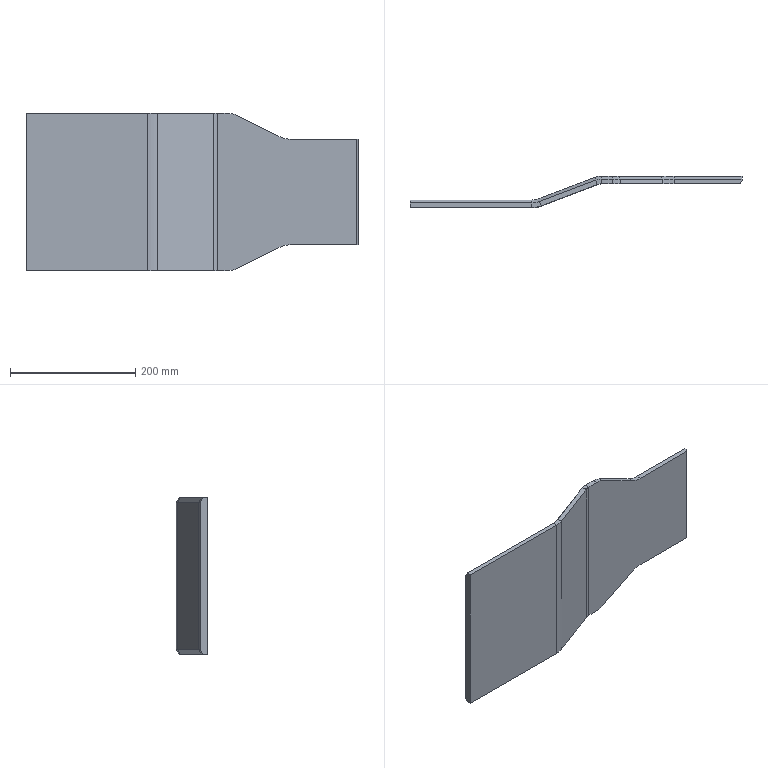Part | SolidWorks | features Chamfer 2, Cut 1, Extrusion 1, FlatPattern 1, SheetMetal 1, SolidToSheetMetal 1 | 1 solid | 49 faces | box 530 x 50 x 251 mm | volume 1438713 mm3 | plane 33 | cylinder 8 | cone 8 | commonest cylinder face diameters 60 x4 80 x2 36 x1 84 x1
STEP:
#1=CARTESIAN_POINT('',(0.,-50.,-10.));
#2=VERTEX_POINT('',#1);
#3=CARTESIAN_POINT('',(0.,-42.619,-10.));
#4=VERTEX_POINT('',#3);
#5=CARTESIAN_POINT('',(0.,-38.,-10.));
#6=DIRECTION('',(0.,1.,0.));
#7=VECTOR('',#6,1000.);
#8=LINE('',#5,#7);
#9=EDGE_CURVE('',#2,#4,#8,.T.);
#10=ORIENTED_EDGE('',*,*,#9,.T.);
#11=CARTESIAN_POINT('',(0.,-38.,-18.));
#12=VERTEX_POINT('',#11);
#13=CARTESIAN_POINT('',(0.,297.738,-599.515));
#14=DIRECTION('',(0.,0.5,-0.866));
#15=VECTOR('',#14,1000.);
#16=LINE('',#13,#15);
#17=EDGE_CURVE('',#4,#12,#16,.T.);
#18=ORIENTED_EDGE('',*,*,#17,.T.);
#19=CARTESIAN_POINT('',(0.,-38.,-253.));
#20=VERTEX_POINT('',#19);
#21=CARTESIAN_POINT('',(0.,-38.,-793.353));
#22=DIRECTION('',(0.,0.,1.));
#23=VECTOR('',#22,1000.);
#24=LINE('',#21,#23);
#25=EDGE_CURVE('',#20,#12,#24,.T.);
#26=ORIENTED_EDGE('',*,*,#25,.F.);
#27=CARTESIAN_POINT('',(0.,-42.619,-261.));
#28=VERTEX_POINT('',#27);
#29=CARTESIAN_POINT('',(0.,-271.98,-658.265));
#30=DIRECTION('',(0.,-0.5,-0.866));
#31=VECTOR('',#30,1000.);
#32=LINE('',#29,#31);
#33=EDGE_CURVE('',#20,#28,#32,.T.);
#34=ORIENTED_EDGE('',*,*,#33,.T.);
#35=CARTESIAN_POINT('',(0.,-50.,-261.));
#36=VERTEX_POINT('',#35);
#37=CARTESIAN_POINT('',(0.,-38.,-261.));
#38=DIRECTION('',(0.,1.,0.));
#39=VECTOR('',#38,1000.);
#40=LINE('',#37,#39);
#41=EDGE_CURVE('',#36,#28,#40,.T.);
#42=ORIENTED_EDGE('',*,*,#41,.F.);
#43=CARTESIAN_POINT('',(0.,-50.,-793.353));
#44=DIRECTION('',(0.,0.,1.));
#45=VECTOR('',#44,1000.);
#46=LINE('',#43,#45);
#47=EDGE_CURVE('',#36,#2,#46,.T.);
#48=ORIENTED_EDGE('',*,*,#47,.T.);
#49=EDGE_LOOP('',(#10,#18,#26,#34,#42,#48));
#50=FACE_OUTER_BOUND('',#49,.T.);
#51=CARTESIAN_POINT('',(0.,-38.,-793.353));
#52=DIRECTION('',(-1.,0.,0.));
#53=DIRECTION('',(0.,0.,1.));
#54=AXIS2_PLACEMENT_3D('',#51,#52,#53);
#55=PLANE('',#54);
#56=ADVANCED_FACE('',(#50),#55,.T.);
#57=CARTESIAN_POINT('',(194.492,-50.,-10.));
#58=VERTEX_POINT('',#57);
#59=CARTESIAN_POINT('',(194.492,-42.619,-10.));
#60=VERTEX_POINT('',#59);
#61=CARTESIAN_POINT('',(194.492,-38.,-10.));
#62=DIRECTION('',(0.,1.,0.));
#63=VECTOR('',#62,1000.);
#64=LINE('',#61,#63);
#65=EDGE_CURVE('',#58,#60,#64,.T.);
#66=ORIENTED_EDGE('',*,*,#65,.T.);
#67=CARTESIAN_POINT('',(0.,-42.619,-10.));
#68=DIRECTION('',(-1.,0.,0.));
#69=VECTOR('',#68,1000.);
#70=LINE('',#67,#69);
#71=EDGE_CURVE('',#60,#4,#70,.T.);
#72=ORIENTED_EDGE('',*,*,#71,.T.);
#73=ORIENTED_EDGE('',*,*,#9,.F.);
#74=CARTESIAN_POINT('',(0.,-50.,-10.));
#75=DIRECTION('',(-1.,0.,0.));
#76=VECTOR('',#75,1000.);
#77=LINE('',#74,#76);
#78=EDGE_CURVE('',#58,#2,#77,.T.);
#79=ORIENTED_EDGE('',*,*,#78,.F.);
#80=EDGE_LOOP('',(#66,#72,#73,#79));
#81=FACE_OUTER_BOUND('',#80,.T.);
#82=CARTESIAN_POINT('',(0.,-38.,-10.));
#83=DIRECTION('',(0.,0.,-1.));
#84=DIRECTION('',(-1.,0.,0.));
#85=AXIS2_PLACEMENT_3D('',#82,#83,#84);
#86=PLANE('',#85);
#87=ADVANCED_FACE('',(#81),#86,.F.);
#88=CARTESIAN_POINT('',(209.411,-47.261,-10.));
#89=VERTEX_POINT('',#88);
#90=CARTESIAN_POINT('',(206.789,-40.361,-10.));
#91=VERTEX_POINT('',#90);
#92=CARTESIAN_POINT('',(205.149,-36.044,-10.));
#93=DIRECTION('',(-0.3552,0.9348,0.));
#94=VECTOR('',#93,1000.);
#95=LINE('',#92,#94);
#96=EDGE_CURVE('',#89,#91,#95,.T.);
#97=ORIENTED_EDGE('',*,*,#96,.T.);
#98=CARTESIAN_POINT('',(194.492,-8.,-10.));
#99=DIRECTION('',(0.,0.,-1.));
#100=DIRECTION('',(1.,0.,0.));
#101=AXIS2_PLACEMENT_3D('',#98,#99,#100);
#102=CIRCLE('',#101,34.619);
#103=EDGE_CURVE('',#91,#60,#102,.T.);
#104=ORIENTED_EDGE('',*,*,#103,.T.);
#105=ORIENTED_EDGE('',*,*,#65,.F.);
#106=CARTESIAN_POINT('',(194.492,-8.,-10.));
#107=DIRECTION('',(0.,0.,-1.));
#108=DIRECTION('',(1.,0.,0.));
#109=AXIS2_PLACEMENT_3D('',#106,#107,#108);
#110=CIRCLE('',#109,42.);
#111=EDGE_CURVE('',#89,#58,#110,.T.);
#112=ORIENTED_EDGE('',*,*,#111,.F.);
#113=EDGE_LOOP('',(#97,#104,#105,#112));
#114=FACE_OUTER_BOUND('',#113,.T.);
#115=CARTESIAN_POINT('',(194.492,-8.,-10.));
#116=DIRECTION('',(0.,0.,1.));
#117=DIRECTION('',(1.,0.,0.));
#118=AXIS2_PLACEMENT_3D('',#115,#116,#117);
#119=PLANE('',#118);
#120=ADVANCED_FACE('',(#114),#119,.T.);
#121=CARTESIAN_POINT('',(299.114,-13.174,-10.));
#122=VERTEX_POINT('',#121);
#123=CARTESIAN_POINT('',(296.492,-6.274,-10.));
#124=VERTEX_POINT('',#123);
#125=CARTESIAN_POINT('',(294.851,-1.956,-10.));
#126=DIRECTION('',(-0.3552,0.9348,0.));
#127=VECTOR('',#126,1000.);
#128=LINE('',#125,#127);
#129=EDGE_CURVE('',#122,#124,#128,.T.);
#130=ORIENTED_EDGE('',*,*,#129,.T.);
#131=CARTESIAN_POINT('',(206.789,-40.361,-10.));
#132=DIRECTION('',(-0.9348,-0.3552,0.));
#133=VECTOR('',#132,1000.);
#134=LINE('',#131,#133);
#135=EDGE_CURVE('',#124,#91,#134,.T.);
#136=ORIENTED_EDGE('',*,*,#135,.T.);
#137=ORIENTED_EDGE('',*,*,#96,.F.);
#138=CARTESIAN_POINT('',(209.411,-47.261,-10.));
#139=DIRECTION('',(-0.9348,-0.3552,0.));
#140=VECTOR('',#139,1000.);
#141=LINE('',#138,#140);
#142=EDGE_CURVE('',#122,#89,#141,.T.);
#143=ORIENTED_EDGE('',*,*,#142,.F.);
#144=EDGE_LOOP('',(#130,#136,#137,#143));
#145=FACE_OUTER_BOUND('',#144,.T.);
#146=CARTESIAN_POINT('',(205.149,-36.044,-10.));
#147=DIRECTION('',(0.,0.,-1.));
#148=DIRECTION('',(-0.9348,-0.3552,0.));
#149=AXIS2_PLACEMENT_3D('',#146,#147,#148);
#150=PLANE('',#149);
#151=ADVANCED_FACE('',(#145),#150,.F.);
#152=CARTESIAN_POINT('',(305.508,-12.,-10.));
#153=VERTEX_POINT('',#152);
#154=CARTESIAN_POINT('',(305.508,-4.619,-10.));
#155=VERTEX_POINT('',#154);
#156=CARTESIAN_POINT('',(305.508,0.,-10.));
#157=DIRECTION('',(0.,1.,0.));
#158=VECTOR('',#157,1000.);
#159=LINE('',#156,#158);
#160=EDGE_CURVE('',#153,#155,#159,.T.);
#161=ORIENTED_EDGE('',*,*,#160,.T.);
#162=CARTESIAN_POINT('',(305.508,-30.,-10.));
#163=DIRECTION('',(0.,0.,1.));
#164=DIRECTION('',(-1.,0.,0.));
#165=AXIS2_PLACEMENT_3D('',#162,#163,#164);
#166=CIRCLE('',#165,25.381);
#167=EDGE_CURVE('',#155,#124,#166,.T.);
#168=ORIENTED_EDGE('',*,*,#167,.T.);
#169=ORIENTED_EDGE('',*,*,#129,.F.);
#170=CARTESIAN_POINT('',(305.508,-30.,-10.));
#171=DIRECTION('',(0.,0.,1.));
#172=DIRECTION('',(1.,0.,0.));
#173=AXIS2_PLACEMENT_3D('',#170,#171,#172);
#174=CIRCLE('',#173,18.);
#175=EDGE_CURVE('',#153,#122,#174,.T.);
#176=ORIENTED_EDGE('',*,*,#175,.F.);
#177=EDGE_LOOP('',(#161,#168,#169,#176));
#178=FACE_OUTER_BOUND('',#177,.T.);
#179=CARTESIAN_POINT('',(305.508,-30.,-10.));
#180=DIRECTION('',(0.,0.,-1.));
#181=DIRECTION('',(-1.,0.,0.));
#182=AXIS2_PLACEMENT_3D('',#179,#180,#181);
#183=PLANE('',#182);
#184=ADVANCED_FACE('',(#178),#183,.F.);
#185=CARTESIAN_POINT('',(322.918,-12.,-10.));
#186=VERTEX_POINT('',#185);
#187=CARTESIAN_POINT('',(322.918,-4.619,-10.));
#188=VERTEX_POINT('',#187);
#189=CARTESIAN_POINT('',(322.918,0.,-10.));
#190=DIRECTION('',(0.,1.,0.));
#191=VECTOR('',#190,1000.);
#192=LINE('',#189,#191);
#193=EDGE_CURVE('',#186,#188,#192,.T.);
#194=ORIENTED_EDGE('',*,*,#193,.T.);
#195=CARTESIAN_POINT('',(322.918,-4.619,-10.));
#196=DIRECTION('',(-1.,0.,0.));
#197=VECTOR('',#196,1000.);
#198=LINE('',#195,#197);
#199=EDGE_CURVE('',#188,#155,#198,.T.);
#200=ORIENTED_EDGE('',*,*,#199,.T.);
#201=ORIENTED_EDGE('',*,*,#160,.F.);
#202=CARTESIAN_POINT('',(322.918,-12.,-10.));
#203=DIRECTION('',(-1.,0.,0.));
#204=VECTOR('',#203,1000.);
#205=LINE('',#202,#204);
#206=EDGE_CURVE('',#186,#153,#205,.T.);
#207=ORIENTED_EDGE('',*,*,#206,.F.);
#208=EDGE_LOOP('',(#194,#200,#201,#207));
#209=FACE_OUTER_BOUND('',#208,.T.);
#210=CARTESIAN_POINT('',(322.918,0.,-10.));
#211=DIRECTION('',(0.,0.,-1.));
#212=DIRECTION('',(-1.,0.,0.));
#213=AXIS2_PLACEMENT_3D('',#210,#211,#212);
#214=PLANE('',#213);
#215=ADVANCED_FACE('',(#209),#214,.F.);
#216=CARTESIAN_POINT('',(336.334,-12.,-13.167));
#217=VERTEX_POINT('',#216);
#218=CARTESIAN_POINT('',(336.334,-4.619,-13.167));
#219=VERTEX_POINT('',#218);
#220=CARTESIAN_POINT('',(336.334,0.,-13.167));
#221=DIRECTION('',(0.,1.,0.));
#222=VECTOR('',#221,1000.);
#223=LINE('',#220,#222);
#224=EDGE_CURVE('',#217,#219,#223,.T.);
#225=ORIENTED_EDGE('',*,*,#224,.T.);
#226=CARTESIAN_POINT('',(322.918,-4.619,-40.));
#227=DIRECTION('',(0.,-1.,0.));
#228=DIRECTION('',(0.,0.,1.));
#229=AXIS2_PLACEMENT_3D('',#226,#227,#228);
#230=CIRCLE('',#229,30.);
#231=EDGE_CURVE('',#219,#188,#230,.T.);
#232=ORIENTED_EDGE('',*,*,#231,.T.);
#233=ORIENTED_EDGE('',*,*,#193,.F.);
#234=CARTESIAN_POINT('',(322.918,-12.,-40.));
#235=DIRECTION('',(0.,-1.,0.));
#236=DIRECTION('',(0.,0.,-1.));
#237=AXIS2_PLACEMENT_3D('',#234,#235,#236);
#238=CIRCLE('',#237,30.);
#239=EDGE_CURVE('',#217,#186,#238,.T.);
#240=ORIENTED_EDGE('',*,*,#239,.F.);
#241=EDGE_LOOP('',(#225,#232,#233,#240));
#242=FACE_OUTER_BOUND('',#241,.T.);
#243=CARTESIAN_POINT('',(322.918,0.,-40.));
#244=DIRECTION('',(0.,1.,0.));
#245=DIRECTION('',(0.,0.,1.));
#246=AXIS2_PLACEMENT_3D('',#243,#244,#245);
#247=CYLINDRICAL_SURFACE('',#246,30.);
#248=ADVANCED_FACE('',(#242),#247,.T.);
#249=CARTESIAN_POINT('',(403.666,-12.,-46.833));
#250=VERTEX_POINT('',#249);
#251=CARTESIAN_POINT('',(403.666,-4.619,-46.833));
#252=VERTEX_POINT('',#251);
#253=CARTESIAN_POINT('',(403.666,0.,-46.833));
#254=DIRECTION('',(0.,1.,0.));
#255=VECTOR('',#254,1000.);
#256=LINE('',#253,#255);
#257=EDGE_CURVE('',#250,#252,#256,.T.);
#258=ORIENTED_EDGE('',*,*,#257,.T.);
#259=CARTESIAN_POINT('',(403.666,-4.619,-46.833));
#260=DIRECTION('',(-0.8944,0.,0.4472));
#261=VECTOR('',#260,1000.);
#262=LINE('',#259,#261);
#263=EDGE_CURVE('',#252,#219,#262,.T.);
#264=ORIENTED_EDGE('',*,*,#263,.T.);
#265=ORIENTED_EDGE('',*,*,#224,.F.);
#266=CARTESIAN_POINT('',(403.666,-12.,-46.833));
#267=DIRECTION('',(-0.8944,0.,0.4472));
#268=VECTOR('',#267,1000.);
#269=LINE('',#266,#268);
#270=EDGE_CURVE('',#250,#217,#269,.T.);
#271=ORIENTED_EDGE('',*,*,#270,.F.);
#272=EDGE_LOOP('',(#258,#264,#265,#271));
#273=FACE_OUTER_BOUND('',#272,.T.);
#274=CARTESIAN_POINT('',(403.666,0.,-46.833));
#275=DIRECTION('',(-0.4472,0.,-0.8944));
#276=DIRECTION('',(-0.8944,0.,0.4472));
#277=AXIS2_PLACEMENT_3D('',#274,#275,#276);
#278=PLANE('',#277);
#279=ADVANCED_FACE('',(#273),#278,.F.);
#280=CARTESIAN_POINT('',(421.554,-12.,-51.056));
#281=VERTEX_POINT('',#280);
#282=CARTESIAN_POINT('',(421.554,-4.619,-51.056));
#283=VERTEX_POINT('',#282);
#284=CARTESIAN_POINT('',(421.554,0.,-51.056));
#285=DIRECTION('',(0.,1.,0.));
#286=VECTOR('',#285,1000.);
#287=LINE('',#284,#286);
#288=EDGE_CURVE('',#281,#283,#287,.T.);
#289=ORIENTED_EDGE('',*,*,#288,.T.);
#290=CARTESIAN_POINT('',(421.554,-4.619,-11.056));
#291=DIRECTION('',(0.,1.,0.));
#292=DIRECTION('',(0.,0.,1.));
#293=AXIS2_PLACEMENT_3D('',#290,#291,#292);
#294=CIRCLE('',#293,40.);
#295=EDGE_CURVE('',#283,#252,#294,.T.);
#296=ORIENTED_EDGE('',*,*,#295,.T.);
#297=ORIENTED_EDGE('',*,*,#257,.F.);
#298=CARTESIAN_POINT('',(421.554,-12.,-11.056));
#299=DIRECTION('',(0.,1.,0.));
#300=DIRECTION('',(0.,0.,1.));
#301=AXIS2_PLACEMENT_3D('',#298,#299,#300);
#302=CIRCLE('',#301,40.);
#303=EDGE_CURVE('',#281,#250,#302,.T.);
#304=ORIENTED_EDGE('',*,*,#303,.F.);
#305=EDGE_LOOP('',(#289,#296,#297,#304));
#306=FACE_OUTER_BOUND('',#305,.T.);
#307=CARTESIAN_POINT('',(421.554,0.,-11.056));
#308=DIRECTION('',(0.,1.,0.));
#309=DIRECTION('',(0.,0.,1.));
#310=AXIS2_PLACEMENT_3D('',#307,#308,#309);
#311=CYLINDRICAL_SURFACE('',#310,40.);
#312=ADVANCED_FACE('',(#306),#311,.F.);
#313=CARTESIAN_POINT('',(527.113,-12.,-51.056));
#314=VERTEX_POINT('',#313);
#315=CARTESIAN_POINT('',(322.918,-12.,-51.056));
#316=DIRECTION('',(-1.,0.,0.));
#317=VECTOR('',#316,1000.);
#318=LINE('',#315,#317);
#319=EDGE_CURVE('',#314,#281,#318,.T.);
#320=ORIENTED_EDGE('',*,*,#319,.F.);
#321=CARTESIAN_POINT('',(530.,-7.,-51.056));
#322=VERTEX_POINT('',#321);
#323=CARTESIAN_POINT('',(533.031,-1.75,-51.056));
#324=DIRECTION('',(0.5,0.866,0.));
#325=VECTOR('',#324,1000.);
#326=LINE('',#323,#325);
#327=EDGE_CURVE('',#314,#322,#326,.T.);
#328=ORIENTED_EDGE('',*,*,#327,.T.);
#329=CARTESIAN_POINT('',(530.,-4.619,-51.056));
#330=VERTEX_POINT('',#329);
#331=CARTESIAN_POINT('',(530.,0.,-51.056));
#332=DIRECTION('',(0.,1.,0.));
#333=VECTOR('',#332,1000.);
#334=LINE('',#331,#333);
#335=EDGE_CURVE('',#322,#330,#334,.T.);
#336=ORIENTED_EDGE('',*,*,#335,.T.);
#337=CARTESIAN_POINT('',(530.,-4.619,-51.056));
#338=DIRECTION('',(-1.,0.,0.));
#339=VECTOR('',#338,1000.);
#340=LINE('',#337,#339);
#341=EDGE_CURVE('',#330,#283,#340,.T.);
#342=ORIENTED_EDGE('',*,*,#341,.T.);
#343=ORIENTED_EDGE('',*,*,#288,.F.);
#344=EDGE_LOOP('',(#320,#328,#336,#342,#343));
#345=FACE_OUTER_BOUND('',#344,.T.);
#346=CARTESIAN_POINT('',(530.,0.,-51.056));
#347=DIRECTION('',(0.,0.,-1.));
#348=DIRECTION('',(-1.,0.,0.));
#349=AXIS2_PLACEMENT_3D('',#346,#347,#348);
#350=PLANE('',#349);
#351=ADVANCED_FACE('',(#345),#350,.F.);
#352=ORIENTED_EDGE('',*,*,#335,.F.);
#353=CARTESIAN_POINT('',(530.,-7.,-219.944));
#354=VERTEX_POINT('',#353);
#355=CARTESIAN_POINT('',(530.,-7.,-219.944));
#356=DIRECTION('',(0.,0.,-1.));
#357=VECTOR('',#356,1000.);
#358=LINE('',#355,#357);
#359=EDGE_CURVE('',#322,#354,#358,.T.);
#360=ORIENTED_EDGE('',*,*,#359,.T.);
#361=CARTESIAN_POINT('',(530.,-4.619,-219.944));
#362=VERTEX_POINT('',#361);
#363=CARTESIAN_POINT('',(530.,0.,-219.944));
#364=DIRECTION('',(0.,1.,0.));
#365=VECTOR('',#364,1000.);
#366=LINE('',#363,#365);
#367=EDGE_CURVE('',#354,#362,#366,.T.);
#368=ORIENTED_EDGE('',*,*,#367,.T.);
#369=CARTESIAN_POINT('',(530.,0.,-211.944));
#370=VERTEX_POINT('',#369);
#371=CARTESIAN_POINT('',(530.,-251.757,-648.001));
#372=DIRECTION('',(0.,0.5,0.866));
#373=VECTOR('',#372,1000.);
#374=LINE('',#371,#373);
#375=EDGE_CURVE('',#362,#370,#374,.T.);
#376=ORIENTED_EDGE('',*,*,#375,.T.);
#377=CARTESIAN_POINT('',(530.,0.,-59.056));
#378=VERTEX_POINT('',#377);
#379=CARTESIAN_POINT('',(530.,0.,-793.353));
#380=DIRECTION('',(0.,0.,1.));
#381=VECTOR('',#380,1000.);
#382=LINE('',#379,#381);
#383=EDGE_CURVE('',#370,#378,#382,.T.);
#384=ORIENTED_EDGE('',*,*,#383,.T.);
#385=CARTESIAN_POINT('',(530.,317.96,-609.779));
#386=DIRECTION('',(0.,-0.5,0.866));
#387=VECTOR('',#386,1000.);
#388=LINE('',#385,#387);
#389=EDGE_CURVE('',#378,#330,#388,.T.);
#390=ORIENTED_EDGE('',*,*,#389,.T.);
#391=EDGE_LOOP('',(#352,#360,#368,#376,#384,#390));
#392=FACE_OUTER_BOUND('',#391,.T.);
#393=CARTESIAN_POINT('',(530.,0.,-793.353));
#394=DIRECTION('',(-1.,0.,0.));
#395=DIRECTION('',(0.,0.,1.));
#396=AXIS2_PLACEMENT_3D('',#393,#394,#395);
#397=PLANE('',#396);
#398=ADVANCED_FACE('',(#392),#397,.F.);
#399=ORIENTED_EDGE('',*,*,#367,.F.);
#400=CARTESIAN_POINT('',(527.113,-12.,-219.944));
#401=VERTEX_POINT('',#400);
#402=CARTESIAN_POINT('',(533.031,-1.75,-219.944));
#403=DIRECTION('',(-0.5,-0.866,0.));
#404=VECTOR('',#403,1000.);
#405=LINE('',#402,#404);
#406=EDGE_CURVE('',#354,#401,#405,.T.);
#407=ORIENTED_EDGE('',*,*,#406,.T.);
#408=CARTESIAN_POINT('',(421.554,-12.,-219.944));
#409=VERTEX_POINT('',#408);
#410=CARTESIAN_POINT('',(322.918,-12.,-219.944));
#411=DIRECTION('',(1.,0.,0.));
#412=VECTOR('',#411,1000.);
#413=LINE('',#410,#412);
#414=EDGE_CURVE('',#409,#401,#413,.T.);
#415=ORIENTED_EDGE('',*,*,#414,.F.);
#416=CARTESIAN_POINT('',(421.554,-4.619,-219.944));
#417=VERTEX_POINT('',#416);
#418=CARTESIAN_POINT('',(421.554,0.,-219.944));
#419=DIRECTION('',(0.,1.,0.));
#420=VECTOR('',#419,1000.);
#421=LINE('',#418,#420);
#422=EDGE_CURVE('',#409,#417,#421,.T.);
#423=ORIENTED_EDGE('',*,*,#422,.T.);
#424=CARTESIAN_POINT('',(530.,-4.619,-219.944));
#425=DIRECTION('',(1.,0.,0.));
#426=VECTOR('',#425,1000.);
#427=LINE('',#424,#426);
#428=EDGE_CURVE('',#417,#362,#427,.T.);
#429=ORIENTED_EDGE('',*,*,#428,.T.);
#430=EDGE_LOOP('',(#399,#407,#415,#423,#429));
#431=FACE_OUTER_BOUND('',#430,.T.);
#432=CARTESIAN_POINT('',(530.,0.,-219.944));
#433=DIRECTION('',(0.,0.,1.));
#434=DIRECTION('',(1.,0.,0.));
#435=AXIS2_PLACEMENT_3D('',#432,#433,#434);
#436=PLANE('',#435);
#437=ADVANCED_FACE('',(#431),#436,.F.);
#438=CARTESIAN_POINT('',(403.666,-12.,-224.167));
#439=VERTEX_POINT('',#438);
#440=CARTESIAN_POINT('',(403.666,-4.619,-224.167));
#441=VERTEX_POINT('',#440);
#442=CARTESIAN_POINT('',(403.666,0.,-224.167));
#443=DIRECTION('',(0.,1.,0.));
#444=VECTOR('',#443,1000.);
#445=LINE('',#442,#444);
#446=EDGE_CURVE('',#439,#441,#445,.T.);
#447=ORIENTED_EDGE('',*,*,#446,.T.);
#448=CARTESIAN_POINT('',(421.554,-4.619,-259.944));
#449=DIRECTION('',(0.,1.,0.));
#450=DIRECTION('',(0.,0.,1.));
#451=AXIS2_PLACEMENT_3D('',#448,#449,#450);
#452=CIRCLE('',#451,40.);
#453=EDGE_CURVE('',#441,#417,#452,.T.);
#454=ORIENTED_EDGE('',*,*,#453,.T.);
#455=ORIENTED_EDGE('',*,*,#422,.F.);
#456=CARTESIAN_POINT('',(421.554,-12.,-259.944));
#457=DIRECTION('',(0.,1.,0.));
#458=DIRECTION('',(0.,0.,1.));
#459=AXIS2_PLACEMENT_3D('',#456,#457,#458);
#460=CIRCLE('',#459,40.);
#461=EDGE_CURVE('',#439,#409,#460,.T.);
#462=ORIENTED_EDGE('',*,*,#461,.F.);
#463=EDGE_LOOP('',(#447,#454,#455,#462));
#464=FACE_OUTER_BOUND('',#463,.T.);
#465=CARTESIAN_POINT('',(421.554,0.,-259.944));
#466=DIRECTION('',(0.,1.,0.));
#467=DIRECTION('',(0.,0.,1.));
#468=AXIS2_PLACEMENT_3D('',#465,#466,#467);
#469=CYLINDRICAL_SURFACE('',#468,40.);
#470=ADVANCED_FACE('',(#464),#469,.F.);
#471=CARTESIAN_POINT('',(336.334,-12.,-257.833));
#472=VERTEX_POINT('',#471);
#473=CARTESIAN_POINT('',(336.334,-4.619,-257.833));
#474=VERTEX_POINT('',#473);
#475=CARTESIAN_POINT('',(336.334,0.,-257.833));
#476=DIRECTION('',(0.,1.,0.));
#477=VECTOR('',#476,1000.);
#478=LINE('',#475,#477);
#479=EDGE_CURVE('',#472,#474,#478,.T.);
#480=ORIENTED_EDGE('',*,*,#479,.T.);
#481=CARTESIAN_POINT('',(403.666,-4.619,-224.167));
#482=DIRECTION('',(0.8944,0.,0.4472));
#483=VECTOR('',#482,1000.);
#484=LINE('',#481,#483);
#485=EDGE_CURVE('',#474,#441,#484,.T.);
#486=ORIENTED_EDGE('',*,*,#485,.T.);
#487=ORIENTED_EDGE('',*,*,#446,.F.);
#488=CARTESIAN_POINT('',(403.666,-12.,-224.167));
#489=DIRECTION('',(0.8944,0.,0.4472));
#490=VECTOR('',#489,1000.);
#491=LINE('',#488,#490);
#492=EDGE_CURVE('',#472,#439,#491,.T.);
#493=ORIENTED_EDGE('',*,*,#492,.F.);
#494=EDGE_LOOP('',(#480,#486,#487,#493));
#495=FACE_OUTER_BOUND('',#494,.T.);
#496=CARTESIAN_POINT('',(403.666,0.,-224.167));
#497=DIRECTION('',(-0.4472,0.,0.8944));
#498=DIRECTION('',(0.8944,0.,0.4472));
#499=AXIS2_PLACEMENT_3D('',#496,#497,#498);
#500=PLANE('',#499);
#501=ADVANCED_FACE('',(#495),#500,.F.);
#502=CARTESIAN_POINT('',(322.918,-12.,-261.));
#503=VERTEX_POINT('',#502);
#504=CARTESIAN_POINT('',(322.918,-4.619,-261.));
#505=VERTEX_POINT('',#504);
#506=CARTESIAN_POINT('',(322.918,0.,-261.));
#507=DIRECTION('',(0.,1.,0.));
#508=VECTOR('',#507,1000.);
#509=LINE('',#506,#508);
#510=EDGE_CURVE('',#503,#505,#509,.T.);
#511=ORIENTED_EDGE('',*,*,#510,.T.);
#512=CARTESIAN_POINT('',(322.918,-4.619,-231.));
#513=DIRECTION('',(0.,-1.,0.));
#514=DIRECTION('',(0.,0.,1.));
#515=AXIS2_PLACEMENT_3D('',#512,#513,#514);
#516=CIRCLE('',#515,30.);
#517=EDGE_CURVE('',#505,#474,#516,.T.);
#518=ORIENTED_EDGE('',*,*,#517,.T.);
#519=ORIENTED_EDGE('',*,*,#479,.F.);
#520=CARTESIAN_POINT('',(322.918,-12.,-231.));
#521=DIRECTION('',(0.,-1.,0.));
#522=DIRECTION('',(0.,0.,-1.));
#523=AXIS2_PLACEMENT_3D('',#520,#521,#522);
#524=CIRCLE('',#523,30.);
#525=EDGE_CURVE('',#503,#472,#524,.T.);
#526=ORIENTED_EDGE('',*,*,#525,.F.);
#527=EDGE_LOOP('',(#511,#518,#519,#526));
#528=FACE_OUTER_BOUND('',#527,.T.);
#529=CARTESIAN_POINT('',(322.918,0.,-231.));
#530=DIRECTION('',(0.,1.,0.));
#531=DIRECTION('',(0.,0.,1.));
#532=AXIS2_PLACEMENT_3D('',#529,#530,#531);
#533=CYLINDRICAL_SURFACE('',#532,30.);
#534=ADVANCED_FACE('',(#528),#533,.T.);
#535=CARTESIAN_POINT('',(305.508,-12.,-261.));
#536=VERTEX_POINT('',#535);
#537=CARTESIAN_POINT('',(305.508,-4.619,-261.));
#538=VERTEX_POINT('',#537);
#539=CARTESIAN_POINT('',(305.508,0.,-261.));
#540=DIRECTION('',(0.,1.,0.));
#541=VECTOR('',#540,1000.);
#542=LINE('',#539,#541);
#543=EDGE_CURVE('',#536,#538,#542,.T.);
#544=ORIENTED_EDGE('',*,*,#543,.T.);
#545=CARTESIAN_POINT('',(322.918,-4.619,-261.));
#546=DIRECTION('',(1.,0.,0.));
#547=VECTOR('',#546,1000.);
#548=LINE('',#545,#547);
#549=EDGE_CURVE('',#538,#505,#548,.T.);
#550=ORIENTED_EDGE('',*,*,#549,.T.);
#551=ORIENTED_EDGE('',*,*,#510,.F.);
#552=CARTESIAN_POINT('',(322.918,-12.,-261.));
#553=DIRECTION('',(1.,0.,0.));
#554=VECTOR('',#553,1000.);
#555=LINE('',#552,#554);
#556=EDGE_CURVE('',#536,#503,#555,.T.);
#557=ORIENTED_EDGE('',*,*,#556,.F.);
#558=EDGE_LOOP('',(#544,#550,#551,#557));
#559=FACE_OUTER_BOUND('',#558,.T.);
#560=CARTESIAN_POINT('',(322.918,0.,-261.));
#561=DIRECTION('',(0.,0.,1.));
#562=DIRECTION('',(1.,0.,0.));
#563=AXIS2_PLACEMENT_3D('',#560,#561,#562);
#564=PLANE('',#563);
#565=ADVANCED_FACE('',(#559),#564,.F.);
#566=CARTESIAN_POINT('',(299.114,-13.174,-261.));
#567=VERTEX_POINT('',#566);
#568=CARTESIAN_POINT('',(296.492,-6.274,-261.));
#569=VERTEX_POINT('',#568);
#570=CARTESIAN_POINT('',(294.851,-1.956,-261.));
#571=DIRECTION('',(-0.3552,0.9348,0.));
#572=VECTOR('',#571,1000.);
#573=LINE('',#570,#572);
#574=EDGE_CURVE('',#567,#569,#573,.T.);
#575=ORIENTED_EDGE('',*,*,#574,.T.);
#576=CARTESIAN_POINT('',(305.508,-30.,-261.));
#577=DIRECTION('',(0.,0.,-1.));
#578=DIRECTION('',(-1.,0.,0.));
#579=AXIS2_PLACEMENT_3D('',#576,#577,#578);
#580=CIRCLE('',#579,25.381);
#581=EDGE_CURVE('',#569,#538,#580,.T.);
#582=ORIENTED_EDGE('',*,*,#581,.T.);
#583=ORIENTED_EDGE('',*,*,#543,.F.);
#584=CARTESIAN_POINT('',(305.508,-30.,-261.));
#585=DIRECTION('',(0.,0.,-1.));
#586=DIRECTION('',(1.,0.,0.));
#587=AXIS2_PLACEMENT_3D('',#584,#585,#586);
#588=CIRCLE('',#587,18.);
#589=EDGE_CURVE('',#567,#536,#588,.T.);
#590=ORIENTED_EDGE('',*,*,#589,.F.);
#591=EDGE_LOOP('',(#575,#582,#583,#590));
#592=FACE_OUTER_BOUND('',#591,.T.);
#593=CARTESIAN_POINT('',(305.508,-30.,-261.));
#594=DIRECTION('',(0.,0.,-1.));
#595=DIRECTION('',(-1.,0.,0.));
#596=AXIS2_PLACEMENT_3D('',#593,#594,#595);
#597=PLANE('',#596);
#598=ADVANCED_FACE('',(#592),#597,.T.);
#599=CARTESIAN_POINT('',(209.411,-47.261,-261.));
#600=VERTEX_POINT('',#599);
#601=CARTESIAN_POINT('',(206.789,-40.361,-261.));
#602=VERTEX_POINT('',#601);
#603=CARTESIAN_POINT('',(205.149,-36.044,-261.));
#604=DIRECTION('',(-0.3552,0.9348,0.));
#605=VECTOR('',#604,1000.);
#606=LINE('',#603,#605);
#607=EDGE_CURVE('',#600,#602,#606,.T.);
#608=ORIENTED_EDGE('',*,*,#607,.T.);
#609=CARTESIAN_POINT('',(206.789,-40.361,-261.));
#610=DIRECTION('',(0.9348,0.3552,0.));
#611=VECTOR('',#610,1000.);
#612=LINE('',#609,#611);
#613=EDGE_CURVE('',#602,#569,#612,.T.);
#614=ORIENTED_EDGE('',*,*,#613,.T.);
#615=ORIENTED_EDGE('',*,*,#574,.F.);
#616=CARTESIAN_POINT('',(209.411,-47.261,-261.));
#617=DIRECTION('',(0.9348,0.3552,0.));
#618=VECTOR('',#617,1000.);
#619=LINE('',#616,#618);
#620=EDGE_CURVE('',#600,#567,#619,.T.);
#621=ORIENTED_EDGE('',*,*,#620,.F.);
#622=EDGE_LOOP('',(#608,#614,#615,#621));
#623=FACE_OUTER_BOUND('',#622,.T.);
#624=CARTESIAN_POINT('',(205.149,-36.044,-261.));
#625=DIRECTION('',(0.,0.,1.));
#626=DIRECTION('',(0.9348,0.3552,0.));
#627=AXIS2_PLACEMENT_3D('',#624,#625,#626);
#628=PLANE('',#627);
#629=ADVANCED_FACE('',(#623),#628,.F.);
#630=CARTESIAN_POINT('',(194.492,-50.,-261.));
#631=VERTEX_POINT('',#630);
#632=CARTESIAN_POINT('',(194.492,-42.619,-261.));
#633=VERTEX_POINT('',#632);
#634=CARTESIAN_POINT('',(194.492,-38.,-261.));
#635=DIRECTION('',(0.,1.,0.));
#636=VECTOR('',#635,1000.);
#637=LINE('',#634,#636);
#638=EDGE_CURVE('',#631,#633,#637,.T.);
#639=ORIENTED_EDGE('',*,*,#638,.T.);
#640=CARTESIAN_POINT('',(194.492,-8.,-261.));
#641=DIRECTION('',(0.,0.,1.));
#642=DIRECTION('',(-1.,0.,0.));
#643=AXIS2_PLACEMENT_3D('',#640,#641,#642);
#644=CIRCLE('',#643,34.619);
#645=EDGE_CURVE('',#633,#602,#644,.T.);
#646=ORIENTED_EDGE('',*,*,#645,.T.);
#647=ORIENTED_EDGE('',*,*,#607,.F.);
#648=CARTESIAN_POINT('',(194.492,-8.,-261.));
#649=DIRECTION('',(0.,0.,1.));
#650=DIRECTION('',(1.,0.,0.));
#651=AXIS2_PLACEMENT_3D('',#648,#649,#650);
#652=CIRCLE('',#651,42.);
#653=EDGE_CURVE('',#631,#600,#652,.T.);
#654=ORIENTED_EDGE('',*,*,#653,.F.);
#655=EDGE_LOOP('',(#639,#646,#647,#654));
#656=FACE_OUTER_BOUND('',#655,.T.);
#657=CARTESIAN_POINT('',(194.492,-8.,-261.));
#658=DIRECTION('',(0.,0.,-1.));
#659=DIRECTION('',(-1.,0.,0.));
#660=AXIS2_PLACEMENT_3D('',#657,#658,#659);
#661=PLANE('',#660);
#662=ADVANCED_FACE('',(#656),#661,.T.);
#663=ORIENTED_EDGE('',*,*,#41,.T.);
#664=CARTESIAN_POINT('',(0.,-42.619,-261.));
#665=DIRECTION('',(1.,0.,0.));
#666=VECTOR('',#665,1000.);
#667=LINE('',#664,#666);
#668=EDGE_CURVE('',#28,#633,#667,.T.);
#669=ORIENTED_EDGE('',*,*,#668,.T.);
#670=ORIENTED_EDGE('',*,*,#638,.F.);
#671=CARTESIAN_POINT('',(0.,-50.,-261.));
#672=DIRECTION('',(1.,0.,0.));
#673=VECTOR('',#672,1000.);
#674=LINE('',#671,#673);
#675=EDGE_CURVE('',#36,#631,#674,.T.);
#676=ORIENTED_EDGE('',*,*,#675,.F.);
#677=EDGE_LOOP('',(#663,#669,#670,#676));
#678=FACE_OUTER_BOUND('',#677,.T.);
#679=CARTESIAN_POINT('',(0.,-38.,-261.));
#680=DIRECTION('',(0.,0.,1.));
#681=DIRECTION('',(1.,0.,0.));
#682=AXIS2_PLACEMENT_3D('',#679,#680,#681);
#683=PLANE('',#682);
#684=ADVANCED_FACE('',(#678),#683,.F.);
#685=CARTESIAN_POINT('',(194.492,-38.,-253.));
#686=VERTEX_POINT('',#685);
#687=CARTESIAN_POINT('',(194.492,-38.,-18.));
#688=VERTEX_POINT('',#687);
#689=CARTESIAN_POINT('',(194.492,-38.,-793.353));
#690=DIRECTION('',(0.,0.,1.));
#691=VECTOR('',#690,1000.);
#692=LINE('',#689,#691);
#693=EDGE_CURVE('',#686,#688,#692,.T.);
#694=ORIENTED_EDGE('',*,*,#693,.T.);
#695=CARTESIAN_POINT('',(205.149,-36.044,-18.));
#696=VERTEX_POINT('',#695);
#697=CARTESIAN_POINT('',(194.492,-8.,-18.));
#698=DIRECTION('',(0.,0.,1.));
#699=DIRECTION('',(1.,0.,0.));
#700=AXIS2_PLACEMENT_3D('',#697,#698,#699);
#701=CIRCLE('',#700,30.);
#702=EDGE_CURVE('',#688,#696,#701,.T.);
#703=ORIENTED_EDGE('',*,*,#702,.T.);
#704=CARTESIAN_POINT('',(205.149,-36.044,-253.));
#705=VERTEX_POINT('',#704);
#706=CARTESIAN_POINT('',(205.149,-36.044,-793.353));
#707=DIRECTION('',(0.,0.,1.));
#708=VECTOR('',#707,1000.);
#709=LINE('',#706,#708);
#710=EDGE_CURVE('',#705,#696,#709,.T.);
#711=ORIENTED_EDGE('',*,*,#710,.F.);
#712=CARTESIAN_POINT('',(194.492,-8.,-253.));
#713=DIRECTION('',(0.,0.,-1.));
#714=DIRECTION('',(-1.,0.,0.));
#715=AXIS2_PLACEMENT_3D('',#712,#713,#714);
#716=CIRCLE('',#715,30.);
#717=EDGE_CURVE('',#705,#686,#716,.T.);
#718=ORIENTED_EDGE('',*,*,#717,.T.);
#719=EDGE_LOOP('',(#694,#703,#711,#718));
#720=FACE_OUTER_BOUND('',#719,.T.);
#721=CARTESIAN_POINT('',(194.492,-8.,-793.353));
#722=DIRECTION('',(0.,0.,1.));
#723=DIRECTION('',(1.,0.,0.));
#724=AXIS2_PLACEMENT_3D('',#721,#722,#723);
#725=CYLINDRICAL_SURFACE('',#724,30.);
#726=ADVANCED_FACE('',(#720),#725,.F.);
#727=ORIENTED_EDGE('',*,*,#25,.T.);
#728=CARTESIAN_POINT('',(0.,-38.,-18.));
#729=DIRECTION('',(1.,0.,0.));
#730=VECTOR('',#729,1000.);
#731=LINE('',#728,#730);
#732=EDGE_CURVE('',#12,#688,#731,.T.);
#733=ORIENTED_EDGE('',*,*,#732,.T.);
#734=ORIENTED_EDGE('',*,*,#693,.F.);
#735=CARTESIAN_POINT('',(0.,-38.,-253.));
#736=DIRECTION('',(-1.,0.,0.));
#737=VECTOR('',#736,1000.);
#738=LINE('',#735,#737);
#739=EDGE_CURVE('',#686,#20,#738,.T.);
#740=ORIENTED_EDGE('',*,*,#739,.T.);
#741=EDGE_LOOP('',(#727,#733,#734,#740));
#742=FACE_OUTER_BOUND('',#741,.T.);
#743=CARTESIAN_POINT('',(0.,-38.,-793.353));
#744=DIRECTION('',(0.,1.,0.));
#745=DIRECTION('',(0.,0.,1.));
#746=AXIS2_PLACEMENT_3D('',#743,#744,#745);
#747=PLANE('',#746);
#748=ADVANCED_FACE('',(#742),#747,.T.);
#749=CARTESIAN_POINT('',(294.851,-1.956,-253.));
#750=VERTEX_POINT('',#749);
#751=CARTESIAN_POINT('',(294.851,-1.956,-18.));
#752=VERTEX_POINT('',#751);
#753=CARTESIAN_POINT('',(294.851,-1.956,-793.353));
#754=DIRECTION('',(0.,0.,1.));
#755=VECTOR('',#754,1000.);
#756=LINE('',#753,#755);
#757=EDGE_CURVE('',#750,#752,#756,.T.);
#758=ORIENTED_EDGE('',*,*,#757,.T.);
#759=CARTESIAN_POINT('',(305.508,0.,-18.));
#760=VERTEX_POINT('',#759);
#761=CARTESIAN_POINT('',(305.508,-30.,-18.));
#762=DIRECTION('',(0.,0.,-1.));
#763=DIRECTION('',(1.,0.,0.));
#764=AXIS2_PLACEMENT_3D('',#761,#762,#763);
#765=CIRCLE('',#764,30.);
#766=EDGE_CURVE('',#752,#760,#765,.T.);
#767=ORIENTED_EDGE('',*,*,#766,.T.);
#768=CARTESIAN_POINT('',(305.508,0.,-253.));
#769=VERTEX_POINT('',#768);
#770=CARTESIAN_POINT('',(305.508,0.,-793.353));
#771=DIRECTION('',(0.,0.,1.));
#772=VECTOR('',#771,1000.);
#773=LINE('',#770,#772);
#774=EDGE_CURVE('',#769,#760,#773,.T.);
#775=ORIENTED_EDGE('',*,*,#774,.F.);
#776=CARTESIAN_POINT('',(305.508,-30.,-253.));
#777=DIRECTION('',(0.,0.,1.));
#778=DIRECTION('',(-1.,0.,0.));
#779=AXIS2_PLACEMENT_3D('',#776,#777,#778);
#780=CIRCLE('',#779,30.);
#781=EDGE_CURVE('',#769,#750,#780,.T.);
#782=ORIENTED_EDGE('',*,*,#781,.T.);
#783=EDGE_LOOP('',(#758,#767,#775,#782));
#784=FACE_OUTER_BOUND('',#783,.T.);
#785=CARTESIAN_POINT('',(305.508,-30.,-793.353));
#786=DIRECTION('',(0.,0.,1.));
#787=DIRECTION('',(1.,0.,0.));
#788=AXIS2_PLACEMENT_3D('',#785,#786,#787);
#789=CYLINDRICAL_SURFACE('',#788,30.);
#790=ADVANCED_FACE('',(#784),#789,.T.);
#791=CARTESIAN_POINT('',(400.088,0.,-53.988));
#792=VERTEX_POINT('',#791);
#793=CARTESIAN_POINT('',(421.554,0.,-59.056));
#794=VERTEX_POINT('',#793);
#795=CARTESIAN_POINT('',(421.554,0.,-11.056));
#796=DIRECTION('',(0.,-1.,0.));
#797=DIRECTION('',(0.,0.,1.));
#798=AXIS2_PLACEMENT_3D('',#795,#796,#797);
#799=CIRCLE('',#798,48.);
#800=EDGE_CURVE('',#792,#794,#799,.T.);
#801=ORIENTED_EDGE('',*,*,#800,.T.);
#802=CARTESIAN_POINT('',(322.918,0.,-59.056));
#803=DIRECTION('',(1.,0.,0.));
#804=VECTOR('',#803,1000.);
#805=LINE('',#802,#804);
#806=EDGE_CURVE('',#794,#378,#805,.T.);
#807=ORIENTED_EDGE('',*,*,#806,.T.);
#808=ORIENTED_EDGE('',*,*,#383,.F.);
#809=CARTESIAN_POINT('',(421.554,0.,-211.944));
#810=VERTEX_POINT('',#809);
#811=CARTESIAN_POINT('',(322.918,0.,-211.944));
#812=DIRECTION('',(-1.,0.,0.));
#813=VECTOR('',#812,1000.);
#814=LINE('',#811,#813);
#815=EDGE_CURVE('',#370,#810,#814,.T.);
#816=ORIENTED_EDGE('',*,*,#815,.T.);
#817=CARTESIAN_POINT('',(400.088,0.,-217.012));
#818=VERTEX_POINT('',#817);
#819=CARTESIAN_POINT('',(421.554,0.,-259.944));
#820=DIRECTION('',(0.,-1.,0.));
#821=DIRECTION('',(0.,0.,1.));
#822=AXIS2_PLACEMENT_3D('',#819,#820,#821);
#823=CIRCLE('',#822,48.);
#824=EDGE_CURVE('',#810,#818,#823,.T.);
#825=ORIENTED_EDGE('',*,*,#824,.T.);
#826=CARTESIAN_POINT('',(332.757,0.,-250.677));
#827=VERTEX_POINT('',#826);
#828=CARTESIAN_POINT('',(107.815,0.,-363.148));
#829=DIRECTION('',(-0.8944,0.,-0.4472));
#830=VECTOR('',#829,1000.);
#831=LINE('',#828,#830);
#832=EDGE_CURVE('',#818,#827,#831,.T.);
#833=ORIENTED_EDGE('',*,*,#832,.T.);
#834=CARTESIAN_POINT('',(322.918,0.,-253.));
#835=VERTEX_POINT('',#834);
#836=CARTESIAN_POINT('',(322.918,0.,-231.));
#837=DIRECTION('',(0.,1.,0.));
#838=DIRECTION('',(0.,0.,1.));
#839=AXIS2_PLACEMENT_3D('',#836,#837,#838);
#840=CIRCLE('',#839,22.);
#841=EDGE_CURVE('',#827,#835,#840,.T.);
#842=ORIENTED_EDGE('',*,*,#841,.T.);
#843=CARTESIAN_POINT('',(322.918,0.,-253.));
#844=DIRECTION('',(-1.,0.,0.));
#845=VECTOR('',#844,1000.);
#846=LINE('',#843,#845);
#847=EDGE_CURVE('',#835,#769,#846,.T.);
#848=ORIENTED_EDGE('',*,*,#847,.T.);
#849=ORIENTED_EDGE('',*,*,#774,.T.);
#850=CARTESIAN_POINT('',(322.918,0.,-18.));
#851=VERTEX_POINT('',#850);
#852=CARTESIAN_POINT('',(322.918,0.,-18.));
#853=DIRECTION('',(1.,0.,0.));
#854=VECTOR('',#853,1000.);
#855=LINE('',#852,#854);
#856=EDGE_CURVE('',#760,#851,#855,.T.);
#857=ORIENTED_EDGE('',*,*,#856,.T.);
#858=CARTESIAN_POINT('',(332.757,0.,-20.323));
#859=VERTEX_POINT('',#858);
#860=CARTESIAN_POINT('',(322.918,0.,-40.));
#861=DIRECTION('',(0.,1.,0.));
#862=DIRECTION('',(0.,0.,1.));
#863=AXIS2_PLACEMENT_3D('',#860,#861,#862);
#864=CIRCLE('',#863,22.);
#865=EDGE_CURVE('',#851,#859,#864,.T.);
#866=ORIENTED_EDGE('',*,*,#865,.T.);
#867=CARTESIAN_POINT('',(634.098,0.,-170.993));
#868=DIRECTION('',(0.8944,0.,-0.4472));
#869=VECTOR('',#868,1000.);
#870=LINE('',#867,#869);
#871=EDGE_CURVE('',#859,#792,#870,.T.);
#872=ORIENTED_EDGE('',*,*,#871,.T.);
#873=EDGE_LOOP('',(#801,#807,#808,#816,#825,#833,#842,#848,#849,#857,#866,#872));
#874=FACE_OUTER_BOUND('',#873,.T.);
#875=CARTESIAN_POINT('',(322.918,0.,-793.353));
#876=DIRECTION('',(0.,1.,0.));
#877=DIRECTION('',(0.,0.,1.));
#878=AXIS2_PLACEMENT_3D('',#875,#876,#877);
#879=PLANE('',#878);
#880=ADVANCED_FACE('',(#874),#879,.T.);
#881=ORIENTED_EDGE('',*,*,#710,.T.);
#882=CARTESIAN_POINT('',(205.149,-36.044,-18.));
#883=DIRECTION('',(0.9348,0.3552,0.));
#884=VECTOR('',#883,1000.);
#885=LINE('',#882,#884);
#886=EDGE_CURVE('',#696,#752,#885,.T.);
#887=ORIENTED_EDGE('',*,*,#886,.T.);
#888=ORIENTED_EDGE('',*,*,#757,.F.);
#889=CARTESIAN_POINT('',(205.149,-36.044,-253.));
#890=DIRECTION('',(-0.9348,-0.3552,0.));
#891=VECTOR('',#890,1000.);
#892=LINE('',#889,#891);
#893=EDGE_CURVE('',#750,#705,#892,.T.);
#894=ORIENTED_EDGE('',*,*,#893,.T.);
#895=EDGE_LOOP('',(#881,#887,#888,#894));
#896=FACE_OUTER_BOUND('',#895,.T.);
#897=CARTESIAN_POINT('',(205.149,-36.044,-793.353));
#898=DIRECTION('',(-0.3552,0.9348,0.));
#899=DIRECTION('',(-0.9348,-0.3552,0.));
#900=AXIS2_PLACEMENT_3D('',#897,#898,#899);
#901=PLANE('',#900);
#902=ADVANCED_FACE('',(#896),#901,.T.);
#903=ORIENTED_EDGE('',*,*,#653,.T.);
#904=CARTESIAN_POINT('',(209.411,-47.261,-793.353));
#905=DIRECTION('',(0.,0.,1.));
#906=VECTOR('',#905,1000.);
#907=LINE('',#904,#906);
#908=EDGE_CURVE('',#600,#89,#907,.T.);
#909=ORIENTED_EDGE('',*,*,#908,.T.);
#910=ORIENTED_EDGE('',*,*,#111,.T.);
#911=CARTESIAN_POINT('',(194.492,-50.,-793.353));
#912=DIRECTION('',(0.,0.,1.));
#913=VECTOR('',#912,1000.);
#914=LINE('',#911,#913);
#915=EDGE_CURVE('',#631,#58,#914,.T.);
#916=ORIENTED_EDGE('',*,*,#915,.F.);
#917=EDGE_LOOP('',(#903,#909,#910,#916));
#918=FACE_OUTER_BOUND('',#917,.T.);
#919=CARTESIAN_POINT('',(194.492,-8.,-793.353));
#920=DIRECTION('',(0.,0.,1.));
#921=DIRECTION('',(1.,0.,0.));
#922=AXIS2_PLACEMENT_3D('',#919,#920,#921);
#923=CYLINDRICAL_SURFACE('',#922,42.);
#924=ADVANCED_FACE('',(#918),#923,.T.);
#925=ORIENTED_EDGE('',*,*,#675,.T.);
#926=ORIENTED_EDGE('',*,*,#915,.T.);
#927=ORIENTED_EDGE('',*,*,#78,.T.);
#928=ORIENTED_EDGE('',*,*,#47,.F.);
#929=EDGE_LOOP('',(#925,#926,#927,#928));
#930=FACE_OUTER_BOUND('',#929,.T.);
#931=CARTESIAN_POINT('',(0.,-50.,-793.353));
#932=DIRECTION('',(0.,1.,0.));
#933=DIRECTION('',(0.,0.,1.));
#934=AXIS2_PLACEMENT_3D('',#931,#932,#933);
#935=PLANE('',#934);
#936=ADVANCED_FACE('',(#930),#935,.F.);
#937=ORIENTED_EDGE('',*,*,#589,.T.);
#938=CARTESIAN_POINT('',(305.508,-12.,-793.353));
#939=DIRECTION('',(0.,0.,1.));
#940=VECTOR('',#939,1000.);
#941=LINE('',#938,#940);
#942=EDGE_CURVE('',#536,#153,#941,.T.);
#943=ORIENTED_EDGE('',*,*,#942,.T.);
#944=ORIENTED_EDGE('',*,*,#175,.T.);
#945=CARTESIAN_POINT('',(299.114,-13.174,-793.353));
#946=DIRECTION('',(0.,0.,1.));
#947=VECTOR('',#946,1000.);
#948=LINE('',#945,#947);
#949=EDGE_CURVE('',#567,#122,#948,.T.);
#950=ORIENTED_EDGE('',*,*,#949,.F.);
#951=EDGE_LOOP('',(#937,#943,#944,#950));
#952=FACE_OUTER_BOUND('',#951,.T.);
#953=CARTESIAN_POINT('',(305.508,-30.,-793.353));
#954=DIRECTION('',(0.,0.,1.));
#955=DIRECTION('',(1.,0.,0.));
#956=AXIS2_PLACEMENT_3D('',#953,#954,#955);
#957=CYLINDRICAL_SURFACE('',#956,18.);
#958=ADVANCED_FACE('',(#952),#957,.F.);
#959=ORIENTED_EDGE('',*,*,#414,.T.);
#960=CARTESIAN_POINT('',(527.113,-12.,-51.056));
#961=DIRECTION('',(0.,0.,1.));
#962=VECTOR('',#961,1000.);
#963=LINE('',#960,#962);
#964=EDGE_CURVE('',#401,#314,#963,.T.);
#965=ORIENTED_EDGE('',*,*,#964,.T.);
#966=ORIENTED_EDGE('',*,*,#319,.T.);
#967=ORIENTED_EDGE('',*,*,#303,.T.);
#968=ORIENTED_EDGE('',*,*,#270,.T.);
#969=ORIENTED_EDGE('',*,*,#239,.T.);
#970=ORIENTED_EDGE('',*,*,#206,.T.);
#971=ORIENTED_EDGE('',*,*,#942,.F.);
#972=ORIENTED_EDGE('',*,*,#556,.T.);
#973=ORIENTED_EDGE('',*,*,#525,.T.);
#974=ORIENTED_EDGE('',*,*,#492,.T.);
#975=ORIENTED_EDGE('',*,*,#461,.T.);
#976=EDGE_LOOP('',(#959,#965,#966,#967,#968,#969,#970,#971,#972,#973,#974,#975));
#977=FACE_OUTER_BOUND('',#976,.T.);
#978=CARTESIAN_POINT('',(322.918,-12.,-793.353));
#979=DIRECTION('',(0.,1.,0.));
#980=DIRECTION('',(0.,0.,1.));
#981=AXIS2_PLACEMENT_3D('',#978,#979,#980);
#982=PLANE('',#981);
#983=ADVANCED_FACE('',(#977),#982,.F.);
#984=ORIENTED_EDGE('',*,*,#620,.T.);
#985=ORIENTED_EDGE('',*,*,#949,.T.);
#986=ORIENTED_EDGE('',*,*,#142,.T.);
#987=ORIENTED_EDGE('',*,*,#908,.F.);
#988=EDGE_LOOP('',(#984,#985,#986,#987));
#989=FACE_OUTER_BOUND('',#988,.T.);
#990=CARTESIAN_POINT('',(209.411,-47.261,-793.353));
#991=DIRECTION('',(-0.3552,0.9348,0.));
#992=DIRECTION('',(-0.9348,-0.3552,0.));
#993=AXIS2_PLACEMENT_3D('',#990,#991,#992);
#994=PLANE('',#993);
#995=ADVANCED_FACE('',(#989),#994,.F.);
#996=ORIENTED_EDGE('',*,*,#17,.F.);
#997=ORIENTED_EDGE('',*,*,#71,.F.);
#998=CARTESIAN_POINT('',(194.492,-38.,-18.));
#999=DIRECTION('',(0.,-0.5,0.866));
#1000=VECTOR('',#999,1000.);
#1001=LINE('',#998,#1000);
#1002=EDGE_CURVE('',#688,#60,#1001,.T.);
#1003=ORIENTED_EDGE('',*,*,#1002,.F.);
#1004=ORIENTED_EDGE('',*,*,#732,.F.);
#1005=EDGE_LOOP('',(#996,#997,#1003,#1004));
#1006=FACE_OUTER_BOUND('',#1005,.T.);
#1007=CARTESIAN_POINT('',(0.,-42.619,-10.));
#1008=DIRECTION('',(0.,0.866,0.5));
#1009=DIRECTION('',(1.,0.,0.));
#1010=AXIS2_PLACEMENT_3D('',#1007,#1008,#1009);
#1011=PLANE('',#1010);
#1012=ADVANCED_FACE('',(#1006),#1011,.T.);
#1013=ORIENTED_EDGE('',*,*,#1002,.T.);
#1014=ORIENTED_EDGE('',*,*,#103,.F.);
#1015=CARTESIAN_POINT('',(205.149,-36.044,-18.));
#1016=DIRECTION('',(0.1776,-0.4674,0.866));
#1017=VECTOR('',#1016,1000.);
#1018=LINE('',#1015,#1017);
#1019=EDGE_CURVE('',#696,#91,#1018,.T.);
#1020=ORIENTED_EDGE('',*,*,#1019,.F.);
#1021=ORIENTED_EDGE('',*,*,#702,.F.);
#1022=EDGE_LOOP('',(#1013,#1014,#1020,#1021));
#1023=FACE_OUTER_BOUND('',#1022,.T.);
#1024=CARTESIAN_POINT('',(194.492,-8.,-10.));
#1025=DIRECTION('',(0.,0.,1.));
#1026=DIRECTION('',(1.,0.,0.));
#1027=AXIS2_PLACEMENT_3D('',#1024,#1025,#1026);
#1028=CONICAL_SURFACE('',#1027,34.619,0.5236);
#1029=ADVANCED_FACE('',(#1023),#1028,.F.);
#1030=ORIENTED_EDGE('',*,*,#1019,.T.);
#1031=ORIENTED_EDGE('',*,*,#135,.F.);
#1032=CARTESIAN_POINT('',(294.851,-1.956,-18.));
#1033=DIRECTION('',(0.1776,-0.4674,0.866));
#1034=VECTOR('',#1033,1000.);
#1035=LINE('',#1032,#1034);
#1036=EDGE_CURVE('',#752,#124,#1035,.T.);
#1037=ORIENTED_EDGE('',*,*,#1036,.F.);
#1038=ORIENTED_EDGE('',*,*,#886,.F.);
#1039=EDGE_LOOP('',(#1030,#1031,#1037,#1038));
#1040=FACE_OUTER_BOUND('',#1039,.T.);
#1041=CARTESIAN_POINT('',(206.789,-40.361,-10.));
#1042=DIRECTION('',(-0.3076,0.8095,0.5));
#1043=DIRECTION('',(0.9348,0.3552,0.));
#1044=AXIS2_PLACEMENT_3D('',#1041,#1042,#1043);
#1045=PLANE('',#1044);
#1046=ADVANCED_FACE('',(#1040),#1045,.T.);
#1047=ORIENTED_EDGE('',*,*,#1036,.T.);
#1048=ORIENTED_EDGE('',*,*,#167,.F.);
#1049=CARTESIAN_POINT('',(305.508,0.,-18.));
#1050=DIRECTION('',(0.,-0.5,0.866));
#1051=VECTOR('',#1050,1000.);
#1052=LINE('',#1049,#1051);
#1053=EDGE_CURVE('',#760,#155,#1052,.T.);
#1054=ORIENTED_EDGE('',*,*,#1053,.F.);
#1055=ORIENTED_EDGE('',*,*,#766,.F.);
#1056=EDGE_LOOP('',(#1047,#1048,#1054,#1055));
#1057=FACE_OUTER_BOUND('',#1056,.T.);
#1058=CARTESIAN_POINT('',(305.508,-30.,-10.));
#1059=DIRECTION('',(0.,0.,-1.));
#1060=DIRECTION('',(-1.,0.,0.));
#1061=AXIS2_PLACEMENT_3D('',#1058,#1059,#1060);
#1062=CONICAL_SURFACE('',#1061,25.381,0.5236);
#1063=ADVANCED_FACE('',(#1057),#1062,.T.);
#1064=ORIENTED_EDGE('',*,*,#1053,.T.);
#1065=ORIENTED_EDGE('',*,*,#199,.F.);
#1066=CARTESIAN_POINT('',(322.918,0.,-18.));
#1067=DIRECTION('',(0.,-0.5,0.866));
#1068=VECTOR('',#1067,1000.);
#1069=LINE('',#1066,#1068);
#1070=EDGE_CURVE('',#851,#188,#1069,.T.);
#1071=ORIENTED_EDGE('',*,*,#1070,.F.);
#1072=ORIENTED_EDGE('',*,*,#856,.F.);
#1073=EDGE_LOOP('',(#1064,#1065,#1071,#1072));
#1074=FACE_OUTER_BOUND('',#1073,.T.);
#1075=CARTESIAN_POINT('',(322.918,-4.619,-10.));
#1076=DIRECTION('',(0.,0.866,0.5));
#1077=DIRECTION('',(1.,0.,0.));
#1078=AXIS2_PLACEMENT_3D('',#1075,#1076,#1077);
#1079=PLANE('',#1078);
#1080=ADVANCED_FACE('',(#1074),#1079,.T.);
#1081=ORIENTED_EDGE('',*,*,#1070,.T.);
#1082=ORIENTED_EDGE('',*,*,#231,.F.);
#1083=CARTESIAN_POINT('',(332.757,0.,-20.323));
#1084=DIRECTION('',(0.3873,-0.5,0.7746));
#1085=VECTOR('',#1084,1000.);
#1086=LINE('',#1083,#1085);
#1087=EDGE_CURVE('',#859,#219,#1086,.T.);
#1088=ORIENTED_EDGE('',*,*,#1087,.F.);
#1089=ORIENTED_EDGE('',*,*,#865,.F.);
#1090=EDGE_LOOP('',(#1081,#1082,#1088,#1089));
#1091=FACE_OUTER_BOUND('',#1090,.T.);
#1092=CARTESIAN_POINT('',(322.918,-4.619,-40.));
#1093=DIRECTION('',(0.,-1.,0.));
#1094=DIRECTION('',(0.,0.,-1.));
#1095=AXIS2_PLACEMENT_3D('',#1092,#1093,#1094);
#1096=CONICAL_SURFACE('',#1095,30.,1.047);
#1097=ADVANCED_FACE('',(#1091),#1096,.T.);
#1098=ORIENTED_EDGE('',*,*,#1087,.T.);
#1099=ORIENTED_EDGE('',*,*,#263,.F.);
#1100=CARTESIAN_POINT('',(400.088,0.,-53.988));
#1101=DIRECTION('',(0.3873,-0.5,0.7746));
#1102=VECTOR('',#1101,1000.);
#1103=LINE('',#1100,#1102);
#1104=EDGE_CURVE('',#792,#252,#1103,.T.);
#1105=ORIENTED_EDGE('',*,*,#1104,.F.);
#1106=ORIENTED_EDGE('',*,*,#871,.F.);
#1107=EDGE_LOOP('',(#1098,#1099,#1105,#1106));
#1108=FACE_OUTER_BOUND('',#1107,.T.);
#1109=CARTESIAN_POINT('',(403.666,-4.619,-46.833));
#1110=DIRECTION('',(0.2236,0.866,0.4472));
#1111=DIRECTION('',(0.8944,0.,-0.4472));
#1112=AXIS2_PLACEMENT_3D('',#1109,#1110,#1111);
#1113=PLANE('',#1112);
#1114=ADVANCED_FACE('',(#1108),#1113,.T.);
#1115=ORIENTED_EDGE('',*,*,#1104,.T.);
#1116=ORIENTED_EDGE('',*,*,#295,.F.);
#1117=CARTESIAN_POINT('',(421.554,0.,-59.056));
#1118=DIRECTION('',(0.,-0.5,0.866));
#1119=VECTOR('',#1118,1000.);
#1120=LINE('',#1117,#1119);
#1121=EDGE_CURVE('',#794,#283,#1120,.T.);
#1122=ORIENTED_EDGE('',*,*,#1121,.F.);
#1123=ORIENTED_EDGE('',*,*,#800,.F.);
#1124=EDGE_LOOP('',(#1115,#1116,#1122,#1123));
#1125=FACE_OUTER_BOUND('',#1124,.T.);
#1126=CARTESIAN_POINT('',(421.554,-4.619,-11.056));
#1127=DIRECTION('',(0.,1.,0.));
#1128=DIRECTION('',(0.,0.,1.));
#1129=AXIS2_PLACEMENT_3D('',#1126,#1127,#1128);
#1130=CONICAL_SURFACE('',#1129,40.,1.047);
#1131=ADVANCED_FACE('',(#1125),#1130,.F.);
#1132=ORIENTED_EDGE('',*,*,#389,.F.);
#1133=ORIENTED_EDGE('',*,*,#806,.F.);
#1134=ORIENTED_EDGE('',*,*,#1121,.T.);
#1135=ORIENTED_EDGE('',*,*,#341,.F.);
#1136=EDGE_LOOP('',(#1132,#1133,#1134,#1135));
#1137=FACE_OUTER_BOUND('',#1136,.T.);
#1138=CARTESIAN_POINT('',(530.,-4.619,-51.056));
#1139=DIRECTION('',(0.,0.866,0.5));
#1140=DIRECTION('',(1.,0.,0.));
#1141=AXIS2_PLACEMENT_3D('',#1138,#1139,#1140);
#1142=PLANE('',#1141);
#1143=ADVANCED_FACE('',(#1137),#1142,.T.);
#1144=ORIENTED_EDGE('',*,*,#33,.F.);
#1145=ORIENTED_EDGE('',*,*,#739,.F.);
#1146=CARTESIAN_POINT('',(194.492,-42.619,-261.));
#1147=DIRECTION('',(0.,0.5,0.866));
#1148=VECTOR('',#1147,1000.);
#1149=LINE('',#1146,#1148);
#1150=EDGE_CURVE('',#633,#686,#1149,.T.);
#1151=ORIENTED_EDGE('',*,*,#1150,.F.);
#1152=ORIENTED_EDGE('',*,*,#668,.F.);
#1153=EDGE_LOOP('',(#1144,#1145,#1151,#1152));
#1154=FACE_OUTER_BOUND('',#1153,.T.);
#1155=CARTESIAN_POINT('',(0.,-42.619,-261.));
#1156=DIRECTION('',(0.,0.866,-0.5));
#1157=DIRECTION('',(-1.,0.,0.));
#1158=AXIS2_PLACEMENT_3D('',#1155,#1156,#1157);
#1159=PLANE('',#1158);
#1160=ADVANCED_FACE('',(#1154),#1159,.T.);
#1161=ORIENTED_EDGE('',*,*,#1150,.T.);
#1162=ORIENTED_EDGE('',*,*,#717,.F.);
#1163=CARTESIAN_POINT('',(206.789,-40.361,-261.));
#1164=DIRECTION('',(-0.1776,0.4674,0.866));
#1165=VECTOR('',#1164,1000.);
#1166=LINE('',#1163,#1165);
#1167=EDGE_CURVE('',#602,#705,#1166,.T.);
#1168=ORIENTED_EDGE('',*,*,#1167,.F.);
#1169=ORIENTED_EDGE('',*,*,#645,.F.);
#1170=EDGE_LOOP('',(#1161,#1162,#1168,#1169));
#1171=FACE_OUTER_BOUND('',#1170,.T.);
#1172=CARTESIAN_POINT('',(194.492,-8.,-261.));
#1173=DIRECTION('',(0.,0.,-1.));
#1174=DIRECTION('',(-1.,0.,0.));
#1175=AXIS2_PLACEMENT_3D('',#1172,#1173,#1174);
#1176=CONICAL_SURFACE('',#1175,34.619,0.5236);
#1177=ADVANCED_FACE('',(#1171),#1176,.F.);
#1178=ORIENTED_EDGE('',*,*,#1167,.T.);
#1179=ORIENTED_EDGE('',*,*,#893,.F.);
#1180=CARTESIAN_POINT('',(296.492,-6.274,-261.));
#1181=DIRECTION('',(-0.1776,0.4674,0.866));
#1182=VECTOR('',#1181,1000.);
#1183=LINE('',#1180,#1182);
#1184=EDGE_CURVE('',#569,#750,#1183,.T.);
#1185=ORIENTED_EDGE('',*,*,#1184,.F.);
#1186=ORIENTED_EDGE('',*,*,#613,.F.);
#1187=EDGE_LOOP('',(#1178,#1179,#1185,#1186));
#1188=FACE_OUTER_BOUND('',#1187,.T.);
#1189=CARTESIAN_POINT('',(206.789,-40.361,-261.));
#1190=DIRECTION('',(-0.3076,0.8095,-0.5));
#1191=DIRECTION('',(-0.9348,-0.3552,0.));
#1192=AXIS2_PLACEMENT_3D('',#1189,#1190,#1191);
#1193=PLANE('',#1192);
#1194=ADVANCED_FACE('',(#1188),#1193,.T.);
#1195=ORIENTED_EDGE('',*,*,#1184,.T.);
#1196=ORIENTED_EDGE('',*,*,#781,.F.);
#1197=CARTESIAN_POINT('',(305.508,-4.619,-261.));
#1198=DIRECTION('',(0.,0.5,0.866));
#1199=VECTOR('',#1198,1000.);
#1200=LINE('',#1197,#1199);
#1201=EDGE_CURVE('',#538,#769,#1200,.T.);
#1202=ORIENTED_EDGE('',*,*,#1201,.F.);
#1203=ORIENTED_EDGE('',*,*,#581,.F.);
#1204=EDGE_LOOP('',(#1195,#1196,#1202,#1203));
#1205=FACE_OUTER_BOUND('',#1204,.T.);
#1206=CARTESIAN_POINT('',(305.508,-30.,-261.));
#1207=DIRECTION('',(0.,0.,1.));
#1208=DIRECTION('',(1.,0.,0.));
#1209=AXIS2_PLACEMENT_3D('',#1206,#1207,#1208);
#1210=CONICAL_SURFACE('',#1209,25.381,0.5236);
#1211=ADVANCED_FACE('',(#1205),#1210,.T.);
#1212=ORIENTED_EDGE('',*,*,#1201,.T.);
#1213=ORIENTED_EDGE('',*,*,#847,.F.);
#1214=CARTESIAN_POINT('',(322.918,-4.619,-261.));
#1215=DIRECTION('',(0.,0.5,0.866));
#1216=VECTOR('',#1215,1000.);
#1217=LINE('',#1214,#1216);
#1218=EDGE_CURVE('',#505,#835,#1217,.T.);
#1219=ORIENTED_EDGE('',*,*,#1218,.F.);
#1220=ORIENTED_EDGE('',*,*,#549,.F.);
#1221=EDGE_LOOP('',(#1212,#1213,#1219,#1220));
#1222=FACE_OUTER_BOUND('',#1221,.T.);
#1223=CARTESIAN_POINT('',(322.918,-4.619,-261.));
#1224=DIRECTION('',(0.,0.866,-0.5));
#1225=DIRECTION('',(-1.,0.,0.));
#1226=AXIS2_PLACEMENT_3D('',#1223,#1224,#1225);
#1227=PLANE('',#1226);
#1228=ADVANCED_FACE('',(#1222),#1227,.T.);
#1229=ORIENTED_EDGE('',*,*,#1218,.T.);
#1230=ORIENTED_EDGE('',*,*,#841,.F.);
#1231=CARTESIAN_POINT('',(336.334,-4.619,-257.833));
#1232=DIRECTION('',(-0.3873,0.5,0.7746));
#1233=VECTOR('',#1232,1000.);
#1234=LINE('',#1231,#1233);
#1235=EDGE_CURVE('',#474,#827,#1234,.T.);
#1236=ORIENTED_EDGE('',*,*,#1235,.F.);
#1237=ORIENTED_EDGE('',*,*,#517,.F.);
#1238=EDGE_LOOP('',(#1229,#1230,#1236,#1237));
#1239=FACE_OUTER_BOUND('',#1238,.T.);
#1240=CARTESIAN_POINT('',(322.918,-4.619,-231.));
#1241=DIRECTION('',(0.,-1.,0.));
#1242=DIRECTION('',(0.,0.,-1.));
#1243=AXIS2_PLACEMENT_3D('',#1240,#1241,#1242);
#1244=CONICAL_SURFACE('',#1243,30.,1.047);
#1245=ADVANCED_FACE('',(#1239),#1244,.T.);
#1246=ORIENTED_EDGE('',*,*,#1235,.T.);
#1247=ORIENTED_EDGE('',*,*,#832,.F.);
#1248=CARTESIAN_POINT('',(403.666,-4.619,-224.167));
#1249=DIRECTION('',(-0.3873,0.5,0.7746));
#1250=VECTOR('',#1249,1000.);
#1251=LINE('',#1248,#1250);
#1252=EDGE_CURVE('',#441,#818,#1251,.T.);
#1253=ORIENTED_EDGE('',*,*,#1252,.F.);
#1254=ORIENTED_EDGE('',*,*,#485,.F.);
#1255=EDGE_LOOP('',(#1246,#1247,#1253,#1254));
#1256=FACE_OUTER_BOUND('',#1255,.T.);
#1257=CARTESIAN_POINT('',(403.666,-4.619,-224.167));
#1258=DIRECTION('',(0.2236,0.866,-0.4472));
#1259=DIRECTION('',(-0.8944,0.,-0.4472));
#1260=AXIS2_PLACEMENT_3D('',#1257,#1258,#1259);
#1261=PLANE('',#1260);
#1262=ADVANCED_FACE('',(#1256),#1261,.T.);
#1263=ORIENTED_EDGE('',*,*,#1252,.T.);
#1264=ORIENTED_EDGE('',*,*,#824,.F.);
#1265=CARTESIAN_POINT('',(421.554,-4.619,-219.944));
#1266=DIRECTION('',(0.,0.5,0.866));
#1267=VECTOR('',#1266,1000.);
#1268=LINE('',#1265,#1267);
#1269=EDGE_CURVE('',#417,#810,#1268,.T.);
#1270=ORIENTED_EDGE('',*,*,#1269,.F.);
#1271=ORIENTED_EDGE('',*,*,#453,.F.);
#1272=EDGE_LOOP('',(#1263,#1264,#1270,#1271));
#1273=FACE_OUTER_BOUND('',#1272,.T.);
#1274=CARTESIAN_POINT('',(421.554,-4.619,-259.944));
#1275=DIRECTION('',(0.,1.,0.));
#1276=DIRECTION('',(0.,0.,1.));
#1277=AXIS2_PLACEMENT_3D('',#1274,#1275,#1276);
#1278=CONICAL_SURFACE('',#1277,40.,1.047);
#1279=ADVANCED_FACE('',(#1273),#1278,.F.);
#1280=ORIENTED_EDGE('',*,*,#1269,.T.);
#1281=ORIENTED_EDGE('',*,*,#815,.F.);
#1282=ORIENTED_EDGE('',*,*,#375,.F.);
#1283=ORIENTED_EDGE('',*,*,#428,.F.);
#1284=EDGE_LOOP('',(#1280,#1281,#1282,#1283));
#1285=FACE_OUTER_BOUND('',#1284,.T.);
#1286=CARTESIAN_POINT('',(530.,-4.619,-219.944));
#1287=DIRECTION('',(0.,0.866,-0.5));
#1288=DIRECTION('',(-1.,0.,0.));
#1289=AXIS2_PLACEMENT_3D('',#1286,#1287,#1288);
#1290=PLANE('',#1289);
#1291=ADVANCED_FACE('',(#1285),#1290,.T.);
#1292=ORIENTED_EDGE('',*,*,#406,.F.);
#1293=ORIENTED_EDGE('',*,*,#359,.F.);
#1294=ORIENTED_EDGE('',*,*,#327,.F.);
#1295=ORIENTED_EDGE('',*,*,#964,.F.);
#1296=EDGE_LOOP('',(#1292,#1293,#1294,#1295));
#1297=FACE_OUTER_BOUND('',#1296,.T.);
#1298=CARTESIAN_POINT('',(527.113,-12.,-793.353));
#1299=DIRECTION('',(-0.866,0.5,0.));
#1300=DIRECTION('',(0.,0.,1.));
#1301=AXIS2_PLACEMENT_3D('',#1298,#1299,#1300);
#1302=PLANE('',#1301);
#1303=ADVANCED_FACE('',(#1297),#1302,.F.);
#1304=CLOSED_SHELL('',(#56,#87,#120,#151,#184,#215,#248,#279,#312,#351,#398,#437,#470,#501,#534,#565,#598,#629,#662,#684,#726,#748,#790,#880,#902,#924,#936,#958,#983,#995,#1012,#1029,#1046,#1063,#1080,#1097,#1114,#1131,#1143,#1160,#1177,#1194,#1211,#1228,#1245,#1262,#1279,#1291,#1303));
#1305=MANIFOLD_SOLID_BREP('',#1304);
#1306=CARTESIAN_POINT('',(0.,0.,0.));
#1307=DIRECTION('',(0.,0.,1.));
#1308=DIRECTION('',(1.,0.,0.));
#1309=AXIS2_PLACEMENT_3D('',#1306,#1307,#1308);
#1310=(LENGTH_UNIT()NAMED_UNIT(*)SI_UNIT(.MILLI.,.METRE.));
#1311=UNCERTAINTY_MEASURE_WITH_UNIT(LENGTH_MEASURE(0.00001),#1310,'','');
#1312=(NAMED_UNIT(*)PLANE_ANGLE_UNIT()SI_UNIT($,.RADIAN.));
#1313=(NAMED_UNIT(*)SI_UNIT($,.STERADIAN.)SOLID_ANGLE_UNIT());
#1314=(GEOMETRIC_REPRESENTATION_CONTEXT(3)GLOBAL_UNCERTAINTY_ASSIGNED_CONTEXT((#1311))GLOBAL_UNIT_ASSIGNED_CONTEXT((#1310,#1312,#1313))REPRESENTATION_CONTEXT('',''));
#1315=ADVANCED_BREP_SHAPE_REPRESENTATION('',(#1305,#1309),#1314);